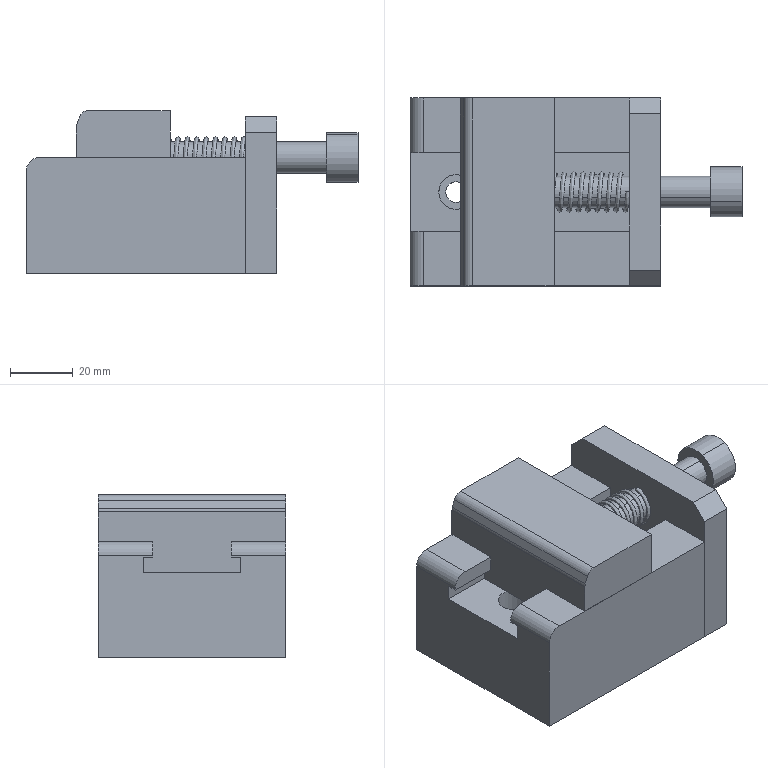Part | SolidWorks | 5 solids | 117 faces | box 106 x 60 x 52 mm | volume 199057 mm3 | cylinder 55 | plane 53 | cone 6 | spline 3 | commonest cylinder face diameters 10.65 x27 11 x6 5 x4 6.5 x4 6.6 x4 6 x2